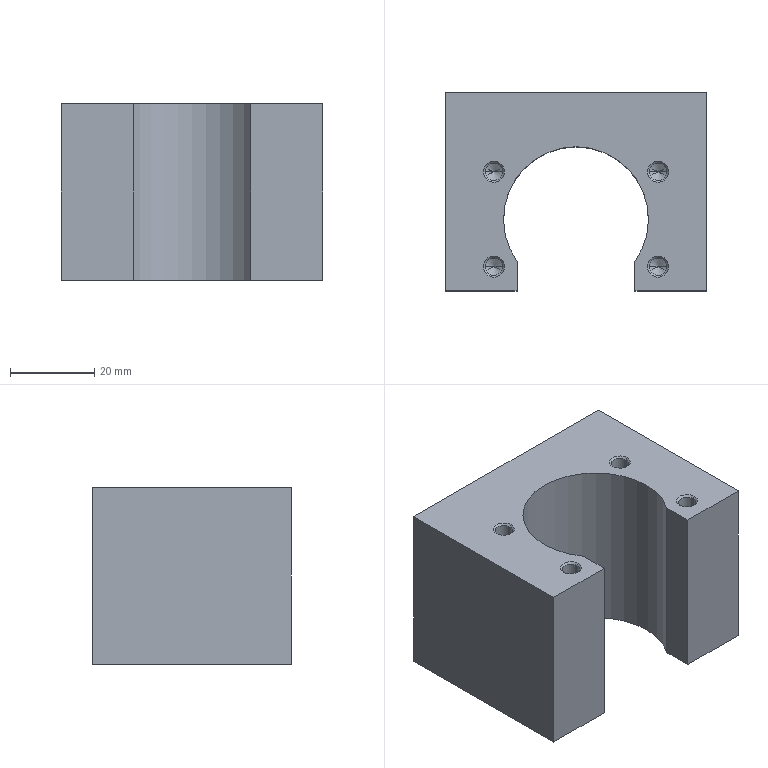Part | SolidWorks | features BaseBody 1 | 1 solid | 58 faces | box 62 x 47 x 42 mm | volume 79435 mm3 | cone 32 | cylinder 17 | plane 9 | commonest cylinder face diameters 4.134 x8 4.917 x8 34.4 x1